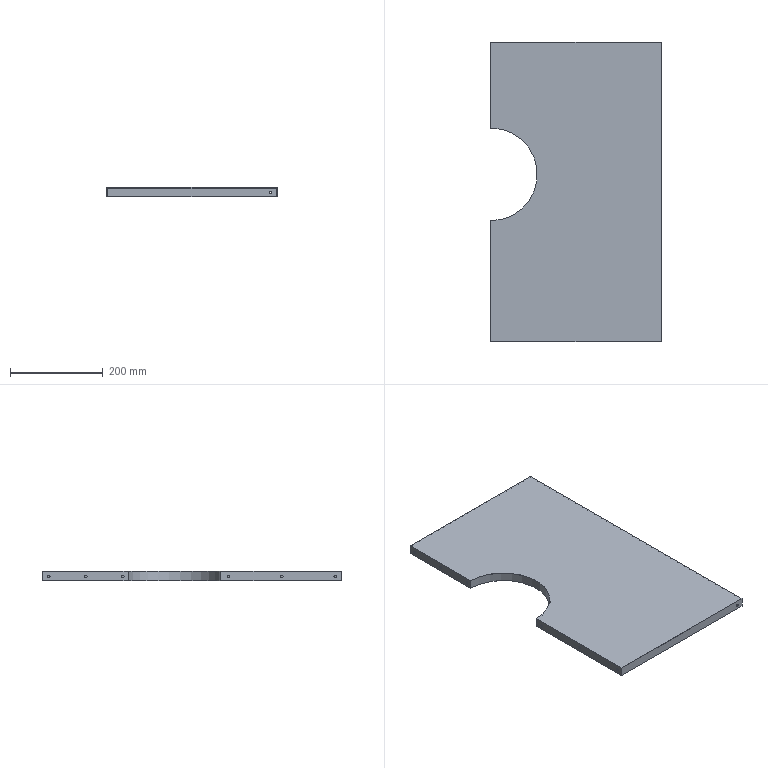Part | SolidWorks | features ICE 2, Extrusion 1, Shell 1 | 1 solid | 31 faces | box 367 x 646 x 20 mm | volume 519095 mm3 | cylinder 18 | plane 13 | commonest cylinder face diameters 5.5 x16 200 x1 204 x1
STEP:
#1=CARTESIAN_POINT('',(0.,244.,11.75));
#2=VERTEX_POINT('',#1);
#3=CARTESIAN_POINT('',(0.,244.,6.25));
#4=VERTEX_POINT('',#3);
#5=CARTESIAN_POINT('',(0.,244.,9.));
#6=DIRECTION('',(1.,0.,0.));
#7=DIRECTION('',(0.,0.,-1.));
#8=AXIS2_PLACEMENT_3D('',#5,#6,#7);
#9=CIRCLE('',#8,2.75);
#10=EDGE_CURVE('',#2,#4,#9,.T.);
#11=ORIENTED_EDGE('',*,*,#10,.F.);
#12=CARTESIAN_POINT('',(2.,244.,11.75));
#13=VERTEX_POINT('',#12);
#14=CARTESIAN_POINT('',(-8.,244.,11.75));
#15=DIRECTION('',(1.,0.,0.));
#16=VECTOR('',#15,1000.);
#17=LINE('',#14,#16);
#18=EDGE_CURVE('',#2,#13,#17,.T.);
#19=ORIENTED_EDGE('',*,*,#18,.T.);
#20=CARTESIAN_POINT('',(2.,244.,6.25));
#21=VERTEX_POINT('',#20);
#22=CARTESIAN_POINT('',(2.,244.,9.));
#23=DIRECTION('',(1.,0.,0.));
#24=DIRECTION('',(0.,0.,-1.));
#25=AXIS2_PLACEMENT_3D('',#22,#23,#24);
#26=CIRCLE('',#25,2.75);
#27=EDGE_CURVE('',#13,#21,#26,.T.);
#28=ORIENTED_EDGE('',*,*,#27,.T.);
#29=CARTESIAN_POINT('',(-8.,244.,6.25));
#30=DIRECTION('',(1.,0.,0.));
#31=VECTOR('',#30,1000.);
#32=LINE('',#29,#31);
#33=EDGE_CURVE('',#4,#21,#32,.T.);
#34=ORIENTED_EDGE('',*,*,#33,.F.);
#35=EDGE_LOOP('',(#11,#19,#28,#34));
#36=FACE_OUTER_BOUND('',#35,.T.);
#37=CARTESIAN_POINT('',(-8.,244.,9.));
#38=DIRECTION('',(1.,0.,0.));
#39=DIRECTION('',(0.,0.,-1.));
#40=AXIS2_PLACEMENT_3D('',#37,#38,#39);
#41=CYLINDRICAL_SURFACE('',#40,2.75);
#42=ADVANCED_FACE('',(#36),#41,.F.);
#43=CARTESIAN_POINT('',(0.,129.,11.75));
#44=VERTEX_POINT('',#43);
#45=CARTESIAN_POINT('',(0.,129.,6.25));
#46=VERTEX_POINT('',#45);
#47=CARTESIAN_POINT('',(0.,129.,9.));
#48=DIRECTION('',(1.,0.,0.));
#49=DIRECTION('',(0.,0.,-1.));
#50=AXIS2_PLACEMENT_3D('',#47,#48,#49);
#51=CIRCLE('',#50,2.75);
#52=EDGE_CURVE('',#44,#46,#51,.T.);
#53=ORIENTED_EDGE('',*,*,#52,.F.);
#54=CARTESIAN_POINT('',(2.,129.,11.75));
#55=VERTEX_POINT('',#54);
#56=CARTESIAN_POINT('',(-8.,129.,11.75));
#57=DIRECTION('',(1.,0.,0.));
#58=VECTOR('',#57,1000.);
#59=LINE('',#56,#58);
#60=EDGE_CURVE('',#44,#55,#59,.T.);
#61=ORIENTED_EDGE('',*,*,#60,.T.);
#62=CARTESIAN_POINT('',(2.,129.,6.25));
#63=VERTEX_POINT('',#62);
#64=CARTESIAN_POINT('',(2.,129.,9.));
#65=DIRECTION('',(1.,0.,0.));
#66=DIRECTION('',(0.,0.,-1.));
#67=AXIS2_PLACEMENT_3D('',#64,#65,#66);
#68=CIRCLE('',#67,2.75);
#69=EDGE_CURVE('',#55,#63,#68,.T.);
#70=ORIENTED_EDGE('',*,*,#69,.T.);
#71=CARTESIAN_POINT('',(-8.,129.,6.25));
#72=DIRECTION('',(1.,0.,0.));
#73=VECTOR('',#72,1000.);
#74=LINE('',#71,#73);
#75=EDGE_CURVE('',#46,#63,#74,.T.);
#76=ORIENTED_EDGE('',*,*,#75,.F.);
#77=EDGE_LOOP('',(#53,#61,#70,#76));
#78=FACE_OUTER_BOUND('',#77,.T.);
#79=CARTESIAN_POINT('',(-8.,129.,9.));
#80=DIRECTION('',(1.,0.,0.));
#81=DIRECTION('',(0.,0.,-1.));
#82=AXIS2_PLACEMENT_3D('',#79,#80,#81);
#83=CYLINDRICAL_SURFACE('',#82,2.75);
#84=ADVANCED_FACE('',(#78),#83,.F.);
#85=CARTESIAN_POINT('',(0.,14.,11.75));
#86=VERTEX_POINT('',#85);
#87=CARTESIAN_POINT('',(0.,14.,6.25));
#88=VERTEX_POINT('',#87);
#89=CARTESIAN_POINT('',(0.,14.,9.));
#90=DIRECTION('',(1.,0.,0.));
#91=DIRECTION('',(0.,0.,-1.));
#92=AXIS2_PLACEMENT_3D('',#89,#90,#91);
#93=CIRCLE('',#92,2.75);
#94=EDGE_CURVE('',#86,#88,#93,.T.);
#95=ORIENTED_EDGE('',*,*,#94,.F.);
#96=CARTESIAN_POINT('',(2.,14.,11.75));
#97=VERTEX_POINT('',#96);
#98=CARTESIAN_POINT('',(-8.,14.,11.75));
#99=DIRECTION('',(1.,0.,0.));
#100=VECTOR('',#99,1000.);
#101=LINE('',#98,#100);
#102=EDGE_CURVE('',#86,#97,#101,.T.);
#103=ORIENTED_EDGE('',*,*,#102,.T.);
#104=CARTESIAN_POINT('',(2.,14.,6.25));
#105=VERTEX_POINT('',#104);
#106=CARTESIAN_POINT('',(2.,14.,9.));
#107=DIRECTION('',(1.,0.,0.));
#108=DIRECTION('',(0.,0.,-1.));
#109=AXIS2_PLACEMENT_3D('',#106,#107,#108);
#110=CIRCLE('',#109,2.75);
#111=EDGE_CURVE('',#97,#105,#110,.T.);
#112=ORIENTED_EDGE('',*,*,#111,.T.);
#113=CARTESIAN_POINT('',(-8.,14.,6.25));
#114=DIRECTION('',(1.,0.,0.));
#115=VECTOR('',#114,1000.);
#116=LINE('',#113,#115);
#117=EDGE_CURVE('',#88,#105,#116,.T.);
#118=ORIENTED_EDGE('',*,*,#117,.F.);
#119=EDGE_LOOP('',(#95,#103,#112,#118));
#120=FACE_OUTER_BOUND('',#119,.T.);
#121=CARTESIAN_POINT('',(-8.,14.,9.));
#122=DIRECTION('',(1.,0.,0.));
#123=DIRECTION('',(0.,0.,-1.));
#124=AXIS2_PLACEMENT_3D('',#121,#122,#123);
#125=CYLINDRICAL_SURFACE('',#124,2.75);
#126=ADVANCED_FACE('',(#120),#125,.F.);
#127=CARTESIAN_POINT('',(0.,472.,11.75));
#128=VERTEX_POINT('',#127);
#129=CARTESIAN_POINT('',(0.,472.,6.25));
#130=VERTEX_POINT('',#129);
#131=CARTESIAN_POINT('',(0.,472.,9.));
#132=DIRECTION('',(1.,0.,0.));
#133=DIRECTION('',(0.,0.,-1.));
#134=AXIS2_PLACEMENT_3D('',#131,#132,#133);
#135=CIRCLE('',#134,2.75);
#136=EDGE_CURVE('',#128,#130,#135,.T.);
#137=ORIENTED_EDGE('',*,*,#136,.F.);
#138=CARTESIAN_POINT('',(2.,472.,11.75));
#139=VERTEX_POINT('',#138);
#140=CARTESIAN_POINT('',(-8.,472.,11.75));
#141=DIRECTION('',(1.,0.,0.));
#142=VECTOR('',#141,1000.);
#143=LINE('',#140,#142);
#144=EDGE_CURVE('',#128,#139,#143,.T.);
#145=ORIENTED_EDGE('',*,*,#144,.T.);
#146=CARTESIAN_POINT('',(2.,472.,6.25));
#147=VERTEX_POINT('',#146);
#148=CARTESIAN_POINT('',(2.,472.,9.));
#149=DIRECTION('',(1.,0.,0.));
#150=DIRECTION('',(0.,0.,-1.));
#151=AXIS2_PLACEMENT_3D('',#148,#149,#150);
#152=CIRCLE('',#151,2.75);
#153=EDGE_CURVE('',#139,#147,#152,.T.);
#154=ORIENTED_EDGE('',*,*,#153,.T.);
#155=CARTESIAN_POINT('',(-8.,472.,6.25));
#156=DIRECTION('',(1.,0.,0.));
#157=VECTOR('',#156,1000.);
#158=LINE('',#155,#157);
#159=EDGE_CURVE('',#130,#147,#158,.T.);
#160=ORIENTED_EDGE('',*,*,#159,.F.);
#161=EDGE_LOOP('',(#137,#145,#154,#160));
#162=FACE_OUTER_BOUND('',#161,.T.);
#163=CARTESIAN_POINT('',(-8.,472.,9.));
#164=DIRECTION('',(1.,0.,0.));
#165=DIRECTION('',(0.,0.,-1.));
#166=AXIS2_PLACEMENT_3D('',#163,#164,#165);
#167=CYLINDRICAL_SURFACE('',#166,2.75);
#168=ADVANCED_FACE('',(#162),#167,.F.);
#169=CARTESIAN_POINT('',(0.,552.,11.75));
#170=VERTEX_POINT('',#169);
#171=CARTESIAN_POINT('',(0.,552.,6.25));
#172=VERTEX_POINT('',#171);
#173=CARTESIAN_POINT('',(0.,552.,9.));
#174=DIRECTION('',(1.,0.,0.));
#175=DIRECTION('',(0.,0.,-1.));
#176=AXIS2_PLACEMENT_3D('',#173,#174,#175);
#177=CIRCLE('',#176,2.75);
#178=EDGE_CURVE('',#170,#172,#177,.T.);
#179=ORIENTED_EDGE('',*,*,#178,.F.);
#180=CARTESIAN_POINT('',(2.,552.,11.75));
#181=VERTEX_POINT('',#180);
#182=CARTESIAN_POINT('',(-8.,552.,11.75));
#183=DIRECTION('',(1.,0.,0.));
#184=VECTOR('',#183,1000.);
#185=LINE('',#182,#184);
#186=EDGE_CURVE('',#170,#181,#185,.T.);
#187=ORIENTED_EDGE('',*,*,#186,.T.);
#188=CARTESIAN_POINT('',(2.,552.,6.25));
#189=VERTEX_POINT('',#188);
#190=CARTESIAN_POINT('',(2.,552.,9.));
#191=DIRECTION('',(1.,0.,0.));
#192=DIRECTION('',(0.,0.,-1.));
#193=AXIS2_PLACEMENT_3D('',#190,#191,#192);
#194=CIRCLE('',#193,2.75);
#195=EDGE_CURVE('',#181,#189,#194,.T.);
#196=ORIENTED_EDGE('',*,*,#195,.T.);
#197=CARTESIAN_POINT('',(-8.,552.,6.25));
#198=DIRECTION('',(1.,0.,0.));
#199=VECTOR('',#198,1000.);
#200=LINE('',#197,#199);
#201=EDGE_CURVE('',#172,#189,#200,.T.);
#202=ORIENTED_EDGE('',*,*,#201,.F.);
#203=EDGE_LOOP('',(#179,#187,#196,#202));
#204=FACE_OUTER_BOUND('',#203,.T.);
#205=CARTESIAN_POINT('',(-8.,552.,9.));
#206=DIRECTION('',(1.,0.,0.));
#207=DIRECTION('',(0.,0.,-1.));
#208=AXIS2_PLACEMENT_3D('',#205,#206,#207);
#209=CYLINDRICAL_SURFACE('',#208,2.75);
#210=ADVANCED_FACE('',(#204),#209,.F.);
#211=CARTESIAN_POINT('',(0.,632.,11.75));
#212=VERTEX_POINT('',#211);
#213=CARTESIAN_POINT('',(0.,632.,6.25));
#214=VERTEX_POINT('',#213);
#215=CARTESIAN_POINT('',(0.,632.,9.));
#216=DIRECTION('',(1.,0.,0.));
#217=DIRECTION('',(0.,0.,-1.));
#218=AXIS2_PLACEMENT_3D('',#215,#216,#217);
#219=CIRCLE('',#218,2.75);
#220=EDGE_CURVE('',#212,#214,#219,.T.);
#221=ORIENTED_EDGE('',*,*,#220,.F.);
#222=CARTESIAN_POINT('',(2.,632.,11.75));
#223=VERTEX_POINT('',#222);
#224=CARTESIAN_POINT('',(-8.,632.,11.75));
#225=DIRECTION('',(1.,0.,0.));
#226=VECTOR('',#225,1000.);
#227=LINE('',#224,#226);
#228=EDGE_CURVE('',#212,#223,#227,.T.);
#229=ORIENTED_EDGE('',*,*,#228,.T.);
#230=CARTESIAN_POINT('',(2.,632.,6.25));
#231=VERTEX_POINT('',#230);
#232=CARTESIAN_POINT('',(2.,632.,9.));
#233=DIRECTION('',(1.,0.,0.));
#234=DIRECTION('',(0.,0.,-1.));
#235=AXIS2_PLACEMENT_3D('',#232,#233,#234);
#236=CIRCLE('',#235,2.75);
#237=EDGE_CURVE('',#223,#231,#236,.T.);
#238=ORIENTED_EDGE('',*,*,#237,.T.);
#239=CARTESIAN_POINT('',(-8.,632.,6.25));
#240=DIRECTION('',(1.,0.,0.));
#241=VECTOR('',#240,1000.);
#242=LINE('',#239,#241);
#243=EDGE_CURVE('',#214,#231,#242,.T.);
#244=ORIENTED_EDGE('',*,*,#243,.F.);
#245=EDGE_LOOP('',(#221,#229,#238,#244));
#246=FACE_OUTER_BOUND('',#245,.T.);
#247=CARTESIAN_POINT('',(-8.,632.,9.));
#248=DIRECTION('',(1.,0.,0.));
#249=DIRECTION('',(0.,0.,-1.));
#250=AXIS2_PLACEMENT_3D('',#247,#248,#249);
#251=CYLINDRICAL_SURFACE('',#250,2.75);
#252=ADVANCED_FACE('',(#246),#251,.F.);
#253=CARTESIAN_POINT('',(353.,2.,11.75));
#254=VERTEX_POINT('',#253);
#255=CARTESIAN_POINT('',(353.,2.,6.25));
#256=VERTEX_POINT('',#255);
#257=CARTESIAN_POINT('',(353.,2.,9.));
#258=DIRECTION('',(0.,-1.,0.));
#259=DIRECTION('',(0.,0.,1.));
#260=AXIS2_PLACEMENT_3D('',#257,#258,#259);
#261=CIRCLE('',#260,2.75);
#262=EDGE_CURVE('',#254,#256,#261,.T.);
#263=ORIENTED_EDGE('',*,*,#262,.F.);
#264=CARTESIAN_POINT('',(353.,0.,11.75));
#265=VERTEX_POINT('',#264);
#266=CARTESIAN_POINT('',(353.,794.,11.75));
#267=DIRECTION('',(0.,-1.,0.));
#268=VECTOR('',#267,1000.);
#269=LINE('',#266,#268);
#270=EDGE_CURVE('',#254,#265,#269,.T.);
#271=ORIENTED_EDGE('',*,*,#270,.T.);
#272=CARTESIAN_POINT('',(353.,0.,6.25));
#273=VERTEX_POINT('',#272);
#274=CARTESIAN_POINT('',(353.,0.,9.));
#275=DIRECTION('',(0.,-1.,0.));
#276=DIRECTION('',(0.,0.,1.));
#277=AXIS2_PLACEMENT_3D('',#274,#275,#276);
#278=CIRCLE('',#277,2.75);
#279=EDGE_CURVE('',#265,#273,#278,.T.);
#280=ORIENTED_EDGE('',*,*,#279,.T.);
#281=CARTESIAN_POINT('',(353.,794.,6.25));
#282=DIRECTION('',(0.,-1.,0.));
#283=VECTOR('',#282,1000.);
#284=LINE('',#281,#283);
#285=EDGE_CURVE('',#256,#273,#284,.T.);
#286=ORIENTED_EDGE('',*,*,#285,.F.);
#287=EDGE_LOOP('',(#263,#271,#280,#286));
#288=FACE_OUTER_BOUND('',#287,.T.);
#289=CARTESIAN_POINT('',(353.,794.,9.));
#290=DIRECTION('',(0.,-1.,0.));
#291=DIRECTION('',(0.,0.,-1.));
#292=AXIS2_PLACEMENT_3D('',#289,#290,#291);
#293=CYLINDRICAL_SURFACE('',#292,2.75);
#294=ADVANCED_FACE('',(#288),#293,.F.);
#295=CARTESIAN_POINT('',(353.,646.,6.25));
#296=VERTEX_POINT('',#295);
#297=CARTESIAN_POINT('',(353.,646.,11.75));
#298=VERTEX_POINT('',#297);
#299=CARTESIAN_POINT('',(353.,646.,9.));
#300=DIRECTION('',(0.,1.,0.));
#301=DIRECTION('',(0.,0.,-1.));
#302=AXIS2_PLACEMENT_3D('',#299,#300,#301);
#303=CIRCLE('',#302,2.75);
#304=EDGE_CURVE('',#296,#298,#303,.T.);
#305=ORIENTED_EDGE('',*,*,#304,.T.);
#306=CARTESIAN_POINT('',(353.,644.,11.75));
#307=VERTEX_POINT('',#306);
#308=CARTESIAN_POINT('',(353.,794.,11.75));
#309=DIRECTION('',(0.,-1.,0.));
#310=VECTOR('',#309,1000.);
#311=LINE('',#308,#310);
#312=EDGE_CURVE('',#298,#307,#311,.T.);
#313=ORIENTED_EDGE('',*,*,#312,.T.);
#314=CARTESIAN_POINT('',(353.,644.,6.25));
#315=VERTEX_POINT('',#314);
#316=CARTESIAN_POINT('',(353.,644.,9.));
#317=DIRECTION('',(0.,1.,0.));
#318=DIRECTION('',(0.,0.,-1.));
#319=AXIS2_PLACEMENT_3D('',#316,#317,#318);
#320=CIRCLE('',#319,2.75);
#321=EDGE_CURVE('',#315,#307,#320,.T.);
#322=ORIENTED_EDGE('',*,*,#321,.F.);
#323=CARTESIAN_POINT('',(353.,794.,6.25));
#324=DIRECTION('',(0.,-1.,0.));
#325=VECTOR('',#324,1000.);
#326=LINE('',#323,#325);
#327=EDGE_CURVE('',#296,#315,#326,.T.);
#328=ORIENTED_EDGE('',*,*,#327,.F.);
#329=EDGE_LOOP('',(#305,#313,#322,#328));
#330=FACE_OUTER_BOUND('',#329,.T.);
#331=CARTESIAN_POINT('',(353.,794.,9.));
#332=DIRECTION('',(0.,-1.,0.));
#333=DIRECTION('',(0.,0.,-1.));
#334=AXIS2_PLACEMENT_3D('',#331,#332,#333);
#335=CYLINDRICAL_SURFACE('',#334,2.75);
#336=ADVANCED_FACE('',(#330),#335,.F.);
#337=CARTESIAN_POINT('',(0.,0.,0.));
#338=VERTEX_POINT('',#337);
#339=CARTESIAN_POINT('',(367.,0.,0.));
#340=VERTEX_POINT('',#339);
#341=CARTESIAN_POINT('',(0.,0.,0.));
#342=DIRECTION('',(1.,0.,0.));
#343=VECTOR('',#342,1000.);
#344=LINE('',#341,#343);
#345=EDGE_CURVE('',#338,#340,#344,.T.);
#346=ORIENTED_EDGE('',*,*,#345,.T.);
#347=CARTESIAN_POINT('',(367.,0.,20.));
#348=VERTEX_POINT('',#347);
#349=CARTESIAN_POINT('',(367.,0.,20.));
#350=DIRECTION('',(0.,0.,-1.));
#351=VECTOR('',#350,1000.);
#352=LINE('',#349,#351);
#353=EDGE_CURVE('',#348,#340,#352,.T.);
#354=ORIENTED_EDGE('',*,*,#353,.F.);
#355=CARTESIAN_POINT('',(0.,0.,20.));
#356=VERTEX_POINT('',#355);
#357=CARTESIAN_POINT('',(0.,0.,20.));
#358=DIRECTION('',(1.,0.,0.));
#359=VECTOR('',#358,1000.);
#360=LINE('',#357,#359);
#361=EDGE_CURVE('',#356,#348,#360,.T.);
#362=ORIENTED_EDGE('',*,*,#361,.F.);
#363=CARTESIAN_POINT('',(0.,0.,20.));
#364=DIRECTION('',(0.,0.,-1.));
#365=VECTOR('',#364,1000.);
#366=LINE('',#363,#365);
#367=EDGE_CURVE('',#356,#338,#366,.T.);
#368=ORIENTED_EDGE('',*,*,#367,.T.);
#369=EDGE_LOOP('',(#346,#354,#362,#368));
#370=FACE_OUTER_BOUND('',#369,.T.);
#371=CARTESIAN_POINT('',(353.,0.,9.));
#372=DIRECTION('',(0.,-1.,0.));
#373=DIRECTION('',(0.,0.,1.));
#374=AXIS2_PLACEMENT_3D('',#371,#372,#373);
#375=CIRCLE('',#374,2.75);
#376=EDGE_CURVE('',#273,#265,#375,.T.);
#377=ORIENTED_EDGE('',*,*,#376,.F.);
#378=ORIENTED_EDGE('',*,*,#279,.F.);
#379=EDGE_LOOP('',(#377,#378));
#380=FACE_BOUND('',#379,.T.);
#381=CARTESIAN_POINT('',(0.,0.,20.));
#382=DIRECTION('',(0.,1.,0.));
#383=DIRECTION('',(0.,0.,1.));
#384=AXIS2_PLACEMENT_3D('',#381,#382,#383);
#385=PLANE('',#384);
#386=ADVANCED_FACE('',(#370,#380),#385,.F.);
#387=CARTESIAN_POINT('',(367.,646.,0.));
#388=VERTEX_POINT('',#387);
#389=CARTESIAN_POINT('',(0.,646.,0.));
#390=VERTEX_POINT('',#389);
#391=CARTESIAN_POINT('',(0.,646.,0.));
#392=DIRECTION('',(-1.,0.,0.));
#393=VECTOR('',#392,1000.);
#394=LINE('',#391,#393);
#395=EDGE_CURVE('',#388,#390,#394,.T.);
#396=ORIENTED_EDGE('',*,*,#395,.T.);
#397=CARTESIAN_POINT('',(0.,646.,20.));
#398=VERTEX_POINT('',#397);
#399=CARTESIAN_POINT('',(0.,646.,20.));
#400=DIRECTION('',(0.,0.,-1.));
#401=VECTOR('',#400,1000.);
#402=LINE('',#399,#401);
#403=EDGE_CURVE('',#398,#390,#402,.T.);
#404=ORIENTED_EDGE('',*,*,#403,.F.);
#405=CARTESIAN_POINT('',(367.,646.,20.));
#406=VERTEX_POINT('',#405);
#407=CARTESIAN_POINT('',(0.,646.,20.));
#408=DIRECTION('',(-1.,0.,0.));
#409=VECTOR('',#408,1000.);
#410=LINE('',#407,#409);
#411=EDGE_CURVE('',#406,#398,#410,.T.);
#412=ORIENTED_EDGE('',*,*,#411,.F.);
#413=CARTESIAN_POINT('',(367.,646.,20.));
#414=DIRECTION('',(0.,0.,-1.));
#415=VECTOR('',#414,1000.);
#416=LINE('',#413,#415);
#417=EDGE_CURVE('',#406,#388,#416,.T.);
#418=ORIENTED_EDGE('',*,*,#417,.T.);
#419=EDGE_LOOP('',(#396,#404,#412,#418));
#420=FACE_OUTER_BOUND('',#419,.T.);
#421=ORIENTED_EDGE('',*,*,#304,.F.);
#422=CARTESIAN_POINT('',(353.,646.,9.));
#423=DIRECTION('',(0.,1.,0.));
#424=DIRECTION('',(0.,0.,-1.));
#425=AXIS2_PLACEMENT_3D('',#422,#423,#424);
#426=CIRCLE('',#425,2.75);
#427=EDGE_CURVE('',#298,#296,#426,.T.);
#428=ORIENTED_EDGE('',*,*,#427,.F.);
#429=EDGE_LOOP('',(#421,#428));
#430=FACE_BOUND('',#429,.T.);
#431=CARTESIAN_POINT('',(0.,646.,20.));
#432=DIRECTION('',(0.,-1.,0.));
#433=DIRECTION('',(0.,0.,-1.));
#434=AXIS2_PLACEMENT_3D('',#431,#432,#433);
#435=PLANE('',#434);
#436=ADVANCED_FACE('',(#420,#430),#435,.F.);
#437=CARTESIAN_POINT('',(2.,2.,0.));
#438=VERTEX_POINT('',#437);
#439=CARTESIAN_POINT('',(365.,2.,0.));
#440=VERTEX_POINT('',#439);
#441=CARTESIAN_POINT('',(0.,2.,0.));
#442=DIRECTION('',(1.,0.,0.));
#443=VECTOR('',#442,1000.);
#444=LINE('',#441,#443);
#445=EDGE_CURVE('',#438,#440,#444,.T.);
#446=ORIENTED_EDGE('',*,*,#445,.F.);
#447=CARTESIAN_POINT('',(2.,2.,18.));
#448=VERTEX_POINT('',#447);
#449=CARTESIAN_POINT('',(2.,2.,20.));
#450=DIRECTION('',(0.,0.,-1.));
#451=VECTOR('',#450,1000.);
#452=LINE('',#449,#451);
#453=EDGE_CURVE('',#448,#438,#452,.T.);
#454=ORIENTED_EDGE('',*,*,#453,.F.);
#455=CARTESIAN_POINT('',(365.,2.,18.));
#456=VERTEX_POINT('',#455);
#457=CARTESIAN_POINT('',(0.,2.,18.));
#458=DIRECTION('',(1.,0.,0.));
#459=VECTOR('',#458,1000.);
#460=LINE('',#457,#459);
#461=EDGE_CURVE('',#448,#456,#460,.T.);
#462=ORIENTED_EDGE('',*,*,#461,.T.);
#463=CARTESIAN_POINT('',(365.,2.,20.));
#464=DIRECTION('',(0.,0.,-1.));
#465=VECTOR('',#464,1000.);
#466=LINE('',#463,#465);
#467=EDGE_CURVE('',#456,#440,#466,.T.);
#468=ORIENTED_EDGE('',*,*,#467,.T.);
#469=EDGE_LOOP('',(#446,#454,#462,#468));
#470=FACE_OUTER_BOUND('',#469,.T.);
#471=CARTESIAN_POINT('',(353.,2.,9.));
#472=DIRECTION('',(0.,-1.,0.));
#473=DIRECTION('',(0.,0.,1.));
#474=AXIS2_PLACEMENT_3D('',#471,#472,#473);
#475=CIRCLE('',#474,2.75);
#476=EDGE_CURVE('',#256,#254,#475,.T.);
#477=ORIENTED_EDGE('',*,*,#476,.T.);
#478=ORIENTED_EDGE('',*,*,#262,.T.);
#479=EDGE_LOOP('',(#477,#478));
#480=FACE_BOUND('',#479,.T.);
#481=CARTESIAN_POINT('',(0.,2.,20.));
#482=DIRECTION('',(0.,1.,0.));
#483=DIRECTION('',(0.,0.,1.));
#484=AXIS2_PLACEMENT_3D('',#481,#482,#483);
#485=PLANE('',#484);
#486=ADVANCED_FACE('',(#470,#480),#485,.T.);
#487=CARTESIAN_POINT('',(365.,644.,0.));
#488=VERTEX_POINT('',#487);
#489=CARTESIAN_POINT('',(2.,644.,0.));
#490=VERTEX_POINT('',#489);
#491=CARTESIAN_POINT('',(0.,644.,0.));
#492=DIRECTION('',(-1.,0.,0.));
#493=VECTOR('',#492,1000.);
#494=LINE('',#491,#493);
#495=EDGE_CURVE('',#488,#490,#494,.T.);
#496=ORIENTED_EDGE('',*,*,#495,.F.);
#497=CARTESIAN_POINT('',(365.,644.,18.));
#498=VERTEX_POINT('',#497);
#499=CARTESIAN_POINT('',(365.,644.,20.));
#500=DIRECTION('',(0.,0.,-1.));
#501=VECTOR('',#500,1000.);
#502=LINE('',#499,#501);
#503=EDGE_CURVE('',#498,#488,#502,.T.);
#504=ORIENTED_EDGE('',*,*,#503,.F.);
#505=CARTESIAN_POINT('',(2.,644.,18.));
#506=VERTEX_POINT('',#505);
#507=CARTESIAN_POINT('',(0.,644.,18.));
#508=DIRECTION('',(-1.,0.,0.));
#509=VECTOR('',#508,1000.);
#510=LINE('',#507,#509);
#511=EDGE_CURVE('',#498,#506,#510,.T.);
#512=ORIENTED_EDGE('',*,*,#511,.T.);
#513=CARTESIAN_POINT('',(2.,644.,20.));
#514=DIRECTION('',(0.,0.,-1.));
#515=VECTOR('',#514,1000.);
#516=LINE('',#513,#515);
#517=EDGE_CURVE('',#506,#490,#516,.T.);
#518=ORIENTED_EDGE('',*,*,#517,.T.);
#519=EDGE_LOOP('',(#496,#504,#512,#518));
#520=FACE_OUTER_BOUND('',#519,.T.);
#521=ORIENTED_EDGE('',*,*,#321,.T.);
#522=CARTESIAN_POINT('',(353.,644.,9.));
#523=DIRECTION('',(0.,1.,0.));
#524=DIRECTION('',(0.,0.,-1.));
#525=AXIS2_PLACEMENT_3D('',#522,#523,#524);
#526=CIRCLE('',#525,2.75);
#527=EDGE_CURVE('',#307,#315,#526,.T.);
#528=ORIENTED_EDGE('',*,*,#527,.T.);
#529=EDGE_LOOP('',(#521,#528));
#530=FACE_BOUND('',#529,.T.);
#531=CARTESIAN_POINT('',(0.,644.,20.));
#532=DIRECTION('',(0.,-1.,0.));
#533=DIRECTION('',(0.,0.,-1.));
#534=AXIS2_PLACEMENT_3D('',#531,#532,#533);
#535=PLANE('',#534);
#536=ADVANCED_FACE('',(#520,#530),#535,.T.);
#537=CARTESIAN_POINT('',(0.,244.,9.));
#538=DIRECTION('',(1.,0.,0.));
#539=DIRECTION('',(0.,0.,-1.));
#540=AXIS2_PLACEMENT_3D('',#537,#538,#539);
#541=CIRCLE('',#540,2.75);
#542=EDGE_CURVE('',#4,#2,#541,.T.);
#543=ORIENTED_EDGE('',*,*,#542,.T.);
#544=ORIENTED_EDGE('',*,*,#10,.T.);
#545=EDGE_LOOP('',(#543,#544));
#546=FACE_BOUND('',#545,.T.);
#547=CARTESIAN_POINT('',(0.,129.,9.));
#548=DIRECTION('',(1.,0.,0.));
#549=DIRECTION('',(0.,0.,-1.));
#550=AXIS2_PLACEMENT_3D('',#547,#548,#549);
#551=CIRCLE('',#550,2.75);
#552=EDGE_CURVE('',#46,#44,#551,.T.);
#553=ORIENTED_EDGE('',*,*,#552,.T.);
#554=ORIENTED_EDGE('',*,*,#52,.T.);
#555=EDGE_LOOP('',(#553,#554));
#556=FACE_BOUND('',#555,.T.);
#557=CARTESIAN_POINT('',(0.,14.,9.));
#558=DIRECTION('',(1.,0.,0.));
#559=DIRECTION('',(0.,0.,-1.));
#560=AXIS2_PLACEMENT_3D('',#557,#558,#559);
#561=CIRCLE('',#560,2.75);
#562=EDGE_CURVE('',#88,#86,#561,.T.);
#563=ORIENTED_EDGE('',*,*,#562,.T.);
#564=ORIENTED_EDGE('',*,*,#94,.T.);
#565=EDGE_LOOP('',(#563,#564));
#566=FACE_BOUND('',#565,.T.);
#567=CARTESIAN_POINT('',(0.,261.,0.));
#568=VERTEX_POINT('',#567);
#569=CARTESIAN_POINT('',(0.,0.,0.));
#570=DIRECTION('',(0.,-1.,0.));
#571=VECTOR('',#570,1000.);
#572=LINE('',#569,#571);
#573=EDGE_CURVE('',#568,#338,#572,.T.);
#574=ORIENTED_EDGE('',*,*,#573,.T.);
#575=ORIENTED_EDGE('',*,*,#367,.F.);
#576=CARTESIAN_POINT('',(0.,261.,20.));
#577=VERTEX_POINT('',#576);
#578=CARTESIAN_POINT('',(0.,0.,20.));
#579=DIRECTION('',(0.,-1.,0.));
#580=VECTOR('',#579,1000.);
#581=LINE('',#578,#580);
#582=EDGE_CURVE('',#577,#356,#581,.T.);
#583=ORIENTED_EDGE('',*,*,#582,.F.);
#584=CARTESIAN_POINT('',(0.,261.,20.));
#585=DIRECTION('',(0.,0.,-1.));
#586=VECTOR('',#585,1000.);
#587=LINE('',#584,#586);
#588=EDGE_CURVE('',#577,#568,#587,.T.);
#589=ORIENTED_EDGE('',*,*,#588,.T.);
#590=EDGE_LOOP('',(#574,#575,#583,#589));
#591=FACE_OUTER_BOUND('',#590,.T.);
#592=CARTESIAN_POINT('',(0.,0.,20.));
#593=DIRECTION('',(1.,0.,0.));
#594=DIRECTION('',(0.,0.,-1.));
#595=AXIS2_PLACEMENT_3D('',#592,#593,#594);
#596=PLANE('',#595);
#597=ADVANCED_FACE('',(#546,#556,#566,#591),#596,.F.);
#598=CARTESIAN_POINT('',(367.,0.,0.));
#599=DIRECTION('',(0.,1.,0.));
#600=VECTOR('',#599,1000.);
#601=LINE('',#598,#600);
#602=EDGE_CURVE('',#340,#388,#601,.T.);
#603=ORIENTED_EDGE('',*,*,#602,.T.);
#604=ORIENTED_EDGE('',*,*,#417,.F.);
#605=CARTESIAN_POINT('',(367.,0.,20.));
#606=DIRECTION('',(0.,1.,0.));
#607=VECTOR('',#606,1000.);
#608=LINE('',#605,#607);
#609=EDGE_CURVE('',#348,#406,#608,.T.);
#610=ORIENTED_EDGE('',*,*,#609,.F.);
#611=ORIENTED_EDGE('',*,*,#353,.T.);
#612=EDGE_LOOP('',(#603,#604,#610,#611));
#613=FACE_OUTER_BOUND('',#612,.T.);
#614=CARTESIAN_POINT('',(367.,0.,20.));
#615=DIRECTION('',(-1.,0.,0.));
#616=DIRECTION('',(0.,0.,1.));
#617=AXIS2_PLACEMENT_3D('',#614,#615,#616);
#618=PLANE('',#617);
#619=ADVANCED_FACE('',(#613),#618,.F.);
#620=CARTESIAN_POINT('',(0.,472.,9.));
#621=DIRECTION('',(1.,0.,0.));
#622=DIRECTION('',(0.,0.,-1.));
#623=AXIS2_PLACEMENT_3D('',#620,#621,#622);
#624=CIRCLE('',#623,2.75);
#625=EDGE_CURVE('',#130,#128,#624,.T.);
#626=ORIENTED_EDGE('',*,*,#625,.T.);
#627=ORIENTED_EDGE('',*,*,#136,.T.);
#628=EDGE_LOOP('',(#626,#627));
#629=FACE_BOUND('',#628,.T.);
#630=CARTESIAN_POINT('',(0.,552.,9.));
#631=DIRECTION('',(1.,0.,0.));
#632=DIRECTION('',(0.,0.,-1.));
#633=AXIS2_PLACEMENT_3D('',#630,#631,#632);
#634=CIRCLE('',#633,2.75);
#635=EDGE_CURVE('',#172,#170,#634,.T.);
#636=ORIENTED_EDGE('',*,*,#635,.T.);
#637=ORIENTED_EDGE('',*,*,#178,.T.);
#638=EDGE_LOOP('',(#636,#637));
#639=FACE_BOUND('',#638,.T.);
#640=CARTESIAN_POINT('',(0.,632.,9.));
#641=DIRECTION('',(1.,0.,0.));
#642=DIRECTION('',(0.,0.,-1.));
#643=AXIS2_PLACEMENT_3D('',#640,#641,#642);
#644=CIRCLE('',#643,2.75);
#645=EDGE_CURVE('',#214,#212,#644,.T.);
#646=ORIENTED_EDGE('',*,*,#645,.T.);
#647=ORIENTED_EDGE('',*,*,#220,.T.);
#648=EDGE_LOOP('',(#646,#647));
#649=FACE_BOUND('',#648,.T.);
#650=CARTESIAN_POINT('',(0.,461.,0.));
#651=VERTEX_POINT('',#650);
#652=CARTESIAN_POINT('',(0.,461.,0.));
#653=DIRECTION('',(0.,-1.,0.));
#654=VECTOR('',#653,1000.);
#655=LINE('',#652,#654);
#656=EDGE_CURVE('',#390,#651,#655,.T.);
#657=ORIENTED_EDGE('',*,*,#656,.T.);
#658=CARTESIAN_POINT('',(0.,461.,20.));
#659=VERTEX_POINT('',#658);
#660=CARTESIAN_POINT('',(0.,461.,20.));
#661=DIRECTION('',(0.,0.,-1.));
#662=VECTOR('',#661,1000.);
#663=LINE('',#660,#662);
#664=EDGE_CURVE('',#659,#651,#663,.T.);
#665=ORIENTED_EDGE('',*,*,#664,.F.);
#666=CARTESIAN_POINT('',(0.,461.,20.));
#667=DIRECTION('',(0.,-1.,0.));
#668=VECTOR('',#667,1000.);
#669=LINE('',#666,#668);
#670=EDGE_CURVE('',#398,#659,#669,.T.);
#671=ORIENTED_EDGE('',*,*,#670,.F.);
#672=ORIENTED_EDGE('',*,*,#403,.T.);
#673=EDGE_LOOP('',(#657,#665,#671,#672));
#674=FACE_OUTER_BOUND('',#673,.T.);
#675=CARTESIAN_POINT('',(0.,461.,20.));
#676=DIRECTION('',(1.,0.,0.));
#677=DIRECTION('',(0.,0.,-1.));
#678=AXIS2_PLACEMENT_3D('',#675,#676,#677);
#679=PLANE('',#678);
#680=ADVANCED_FACE('',(#629,#639,#649,#674),#679,.F.);
#681=CARTESIAN_POINT('',(0.,361.,0.));
#682=DIRECTION('',(0.,0.,-1.));
#683=DIRECTION('',(1.,0.,0.));
#684=AXIS2_PLACEMENT_3D('',#681,#682,#683);
#685=CIRCLE('',#684,100.);
#686=EDGE_CURVE('',#651,#568,#685,.T.);
#687=ORIENTED_EDGE('',*,*,#686,.T.);
#688=ORIENTED_EDGE('',*,*,#588,.F.);
#689=CARTESIAN_POINT('',(0.,361.,20.));
#690=DIRECTION('',(0.,0.,-1.));
#691=DIRECTION('',(1.,0.,0.));
#692=AXIS2_PLACEMENT_3D('',#689,#690,#691);
#693=CIRCLE('',#692,100.);
#694=EDGE_CURVE('',#659,#577,#693,.T.);
#695=ORIENTED_EDGE('',*,*,#694,.F.);
#696=ORIENTED_EDGE('',*,*,#664,.T.);
#697=EDGE_LOOP('',(#687,#688,#695,#696));
#698=FACE_OUTER_BOUND('',#697,.T.);
#699=CARTESIAN_POINT('',(0.,361.,20.));
#700=DIRECTION('',(0.,0.,-1.));
#701=DIRECTION('',(-1.,0.,0.));
#702=AXIS2_PLACEMENT_3D('',#699,#700,#701);
#703=CYLINDRICAL_SURFACE('',#702,100.);
#704=ADVANCED_FACE('',(#698),#703,.F.);
#705=ORIENTED_EDGE('',*,*,#582,.T.);
#706=ORIENTED_EDGE('',*,*,#361,.T.);
#707=ORIENTED_EDGE('',*,*,#609,.T.);
#708=ORIENTED_EDGE('',*,*,#411,.T.);
#709=ORIENTED_EDGE('',*,*,#670,.T.);
#710=ORIENTED_EDGE('',*,*,#694,.T.);
#711=EDGE_LOOP('',(#705,#706,#707,#708,#709,#710));
#712=FACE_OUTER_BOUND('',#711,.T.);
#713=CARTESIAN_POINT('',(0.,361.,20.));
#714=DIRECTION('',(0.,0.,1.));
#715=DIRECTION('',(1.,0.,0.));
#716=AXIS2_PLACEMENT_3D('',#713,#714,#715);
#717=PLANE('',#716);
#718=ADVANCED_FACE('',(#712),#717,.T.);
#719=CARTESIAN_POINT('',(2.,462.98,0.));
#720=VERTEX_POINT('',#719);
#721=CARTESIAN_POINT('',(2.,259.02,0.));
#722=VERTEX_POINT('',#721);
#723=CARTESIAN_POINT('',(0.,361.,0.));
#724=DIRECTION('',(0.,0.,-1.));
#725=DIRECTION('',(1.,0.,0.));
#726=AXIS2_PLACEMENT_3D('',#723,#724,#725);
#727=CIRCLE('',#726,102.);
#728=EDGE_CURVE('',#720,#722,#727,.T.);
#729=ORIENTED_EDGE('',*,*,#728,.T.);
#730=CARTESIAN_POINT('',(2.,0.,0.));
#731=DIRECTION('',(0.,-1.,0.));
#732=VECTOR('',#731,1000.);
#733=LINE('',#730,#732);
#734=EDGE_CURVE('',#722,#438,#733,.T.);
#735=ORIENTED_EDGE('',*,*,#734,.T.);
#736=ORIENTED_EDGE('',*,*,#445,.T.);
#737=CARTESIAN_POINT('',(365.,0.,0.));
#738=DIRECTION('',(0.,1.,0.));
#739=VECTOR('',#738,1000.);
#740=LINE('',#737,#739);
#741=EDGE_CURVE('',#440,#488,#740,.T.);
#742=ORIENTED_EDGE('',*,*,#741,.T.);
#743=ORIENTED_EDGE('',*,*,#495,.T.);
#744=CARTESIAN_POINT('',(2.,461.,0.));
#745=DIRECTION('',(0.,-1.,0.));
#746=VECTOR('',#745,1000.);
#747=LINE('',#744,#746);
#748=EDGE_CURVE('',#490,#720,#747,.T.);
#749=ORIENTED_EDGE('',*,*,#748,.T.);
#750=EDGE_LOOP('',(#729,#735,#736,#742,#743,#749));
#751=FACE_BOUND('',#750,.T.);
#752=ORIENTED_EDGE('',*,*,#573,.F.);
#753=ORIENTED_EDGE('',*,*,#686,.F.);
#754=ORIENTED_EDGE('',*,*,#656,.F.);
#755=ORIENTED_EDGE('',*,*,#395,.F.);
#756=ORIENTED_EDGE('',*,*,#602,.F.);
#757=ORIENTED_EDGE('',*,*,#345,.F.);
#758=EDGE_LOOP('',(#752,#753,#754,#755,#756,#757));
#759=FACE_OUTER_BOUND('',#758,.T.);
#760=CARTESIAN_POINT('',(0.,361.,0.));
#761=DIRECTION('',(0.,0.,1.));
#762=DIRECTION('',(1.,0.,0.));
#763=AXIS2_PLACEMENT_3D('',#760,#761,#762);
#764=PLANE('',#763);
#765=ADVANCED_FACE('',(#751,#759),#764,.F.);
#766=CARTESIAN_POINT('',(2.,244.,9.));
#767=DIRECTION('',(1.,0.,0.));
#768=DIRECTION('',(0.,0.,-1.));
#769=AXIS2_PLACEMENT_3D('',#766,#767,#768);
#770=CIRCLE('',#769,2.75);
#771=EDGE_CURVE('',#21,#13,#770,.T.);
#772=ORIENTED_EDGE('',*,*,#771,.F.);
#773=ORIENTED_EDGE('',*,*,#27,.F.);
#774=EDGE_LOOP('',(#772,#773));
#775=FACE_BOUND('',#774,.T.);
#776=CARTESIAN_POINT('',(2.,129.,9.));
#777=DIRECTION('',(1.,0.,0.));
#778=DIRECTION('',(0.,0.,-1.));
#779=AXIS2_PLACEMENT_3D('',#776,#777,#778);
#780=CIRCLE('',#779,2.75);
#781=EDGE_CURVE('',#63,#55,#780,.T.);
#782=ORIENTED_EDGE('',*,*,#781,.F.);
#783=ORIENTED_EDGE('',*,*,#69,.F.);
#784=EDGE_LOOP('',(#782,#783));
#785=FACE_BOUND('',#784,.T.);
#786=CARTESIAN_POINT('',(2.,14.,9.));
#787=DIRECTION('',(1.,0.,0.));
#788=DIRECTION('',(0.,0.,-1.));
#789=AXIS2_PLACEMENT_3D('',#786,#787,#788);
#790=CIRCLE('',#789,2.75);
#791=EDGE_CURVE('',#105,#97,#790,.T.);
#792=ORIENTED_EDGE('',*,*,#791,.F.);
#793=ORIENTED_EDGE('',*,*,#111,.F.);
#794=EDGE_LOOP('',(#792,#793));
#795=FACE_BOUND('',#794,.T.);
#796=ORIENTED_EDGE('',*,*,#734,.F.);
#797=CARTESIAN_POINT('',(2.,259.02,18.));
#798=VERTEX_POINT('',#797);
#799=CARTESIAN_POINT('',(2.,259.02,18.));
#800=DIRECTION('',(0.,0.,-1.));
#801=VECTOR('',#800,1000.);
#802=LINE('',#799,#801);
#803=EDGE_CURVE('',#798,#722,#802,.T.);
#804=ORIENTED_EDGE('',*,*,#803,.F.);
#805=CARTESIAN_POINT('',(2.,0.,18.));
#806=DIRECTION('',(0.,-1.,0.));
#807=VECTOR('',#806,1000.);
#808=LINE('',#805,#807);
#809=EDGE_CURVE('',#798,#448,#808,.T.);
#810=ORIENTED_EDGE('',*,*,#809,.T.);
#811=ORIENTED_EDGE('',*,*,#453,.T.);
#812=EDGE_LOOP('',(#796,#804,#810,#811));
#813=FACE_OUTER_BOUND('',#812,.T.);
#814=CARTESIAN_POINT('',(2.,0.,20.));
#815=DIRECTION('',(1.,0.,0.));
#816=DIRECTION('',(0.,0.,-1.));
#817=AXIS2_PLACEMENT_3D('',#814,#815,#816);
#818=PLANE('',#817);
#819=ADVANCED_FACE('',(#775,#785,#795,#813),#818,.T.);
#820=ORIENTED_EDGE('',*,*,#741,.F.);
#821=ORIENTED_EDGE('',*,*,#467,.F.);
#822=CARTESIAN_POINT('',(365.,0.,18.));
#823=DIRECTION('',(0.,1.,0.));
#824=VECTOR('',#823,1000.);
#825=LINE('',#822,#824);
#826=EDGE_CURVE('',#456,#498,#825,.T.);
#827=ORIENTED_EDGE('',*,*,#826,.T.);
#828=ORIENTED_EDGE('',*,*,#503,.T.);
#829=EDGE_LOOP('',(#820,#821,#827,#828));
#830=FACE_OUTER_BOUND('',#829,.T.);
#831=CARTESIAN_POINT('',(365.,0.,20.));
#832=DIRECTION('',(-1.,0.,0.));
#833=DIRECTION('',(0.,0.,1.));
#834=AXIS2_PLACEMENT_3D('',#831,#832,#833);
#835=PLANE('',#834);
#836=ADVANCED_FACE('',(#830),#835,.T.);
#837=CARTESIAN_POINT('',(2.,472.,9.));
#838=DIRECTION('',(1.,0.,0.));
#839=DIRECTION('',(0.,0.,-1.));
#840=AXIS2_PLACEMENT_3D('',#837,#838,#839);
#841=CIRCLE('',#840,2.75);
#842=EDGE_CURVE('',#147,#139,#841,.T.);
#843=ORIENTED_EDGE('',*,*,#842,.F.);
#844=ORIENTED_EDGE('',*,*,#153,.F.);
#845=EDGE_LOOP('',(#843,#844));
#846=FACE_BOUND('',#845,.T.);
#847=CARTESIAN_POINT('',(2.,552.,9.));
#848=DIRECTION('',(1.,0.,0.));
#849=DIRECTION('',(0.,0.,-1.));
#850=AXIS2_PLACEMENT_3D('',#847,#848,#849);
#851=CIRCLE('',#850,2.75);
#852=EDGE_CURVE('',#189,#181,#851,.T.);
#853=ORIENTED_EDGE('',*,*,#852,.F.);
#854=ORIENTED_EDGE('',*,*,#195,.F.);
#855=EDGE_LOOP('',(#853,#854));
#856=FACE_BOUND('',#855,.T.);
#857=CARTESIAN_POINT('',(2.,632.,9.));
#858=DIRECTION('',(1.,0.,0.));
#859=DIRECTION('',(0.,0.,-1.));
#860=AXIS2_PLACEMENT_3D('',#857,#858,#859);
#861=CIRCLE('',#860,2.75);
#862=EDGE_CURVE('',#231,#223,#861,.T.);
#863=ORIENTED_EDGE('',*,*,#862,.F.);
#864=ORIENTED_EDGE('',*,*,#237,.F.);
#865=EDGE_LOOP('',(#863,#864));
#866=FACE_BOUND('',#865,.T.);
#867=ORIENTED_EDGE('',*,*,#748,.F.);
#868=ORIENTED_EDGE('',*,*,#517,.F.);
#869=CARTESIAN_POINT('',(2.,462.98,18.));
#870=VERTEX_POINT('',#869);
#871=CARTESIAN_POINT('',(2.,461.,18.));
#872=DIRECTION('',(0.,-1.,0.));
#873=VECTOR('',#872,1000.);
#874=LINE('',#871,#873);
#875=EDGE_CURVE('',#506,#870,#874,.T.);
#876=ORIENTED_EDGE('',*,*,#875,.T.);
#877=CARTESIAN_POINT('',(2.,462.98,18.));
#878=DIRECTION('',(0.,0.,-1.));
#879=VECTOR('',#878,1000.);
#880=LINE('',#877,#879);
#881=EDGE_CURVE('',#870,#720,#880,.T.);
#882=ORIENTED_EDGE('',*,*,#881,.T.);
#883=EDGE_LOOP('',(#867,#868,#876,#882));
#884=FACE_OUTER_BOUND('',#883,.T.);
#885=CARTESIAN_POINT('',(2.,461.,20.));
#886=DIRECTION('',(1.,0.,0.));
#887=DIRECTION('',(0.,0.,-1.));
#888=AXIS2_PLACEMENT_3D('',#885,#886,#887);
#889=PLANE('',#888);
#890=ADVANCED_FACE('',(#846,#856,#866,#884),#889,.T.);
#891=ORIENTED_EDGE('',*,*,#728,.F.);
#892=ORIENTED_EDGE('',*,*,#881,.F.);
#893=CARTESIAN_POINT('',(0.,361.,18.));
#894=DIRECTION('',(0.,0.,-1.));
#895=DIRECTION('',(1.,0.,0.));
#896=AXIS2_PLACEMENT_3D('',#893,#894,#895);
#897=CIRCLE('',#896,102.);
#898=EDGE_CURVE('',#870,#798,#897,.T.);
#899=ORIENTED_EDGE('',*,*,#898,.T.);
#900=ORIENTED_EDGE('',*,*,#803,.T.);
#901=EDGE_LOOP('',(#891,#892,#899,#900));
#902=FACE_OUTER_BOUND('',#901,.T.);
#903=CARTESIAN_POINT('',(0.,361.,20.));
#904=DIRECTION('',(0.,0.,-1.));
#905=DIRECTION('',(-1.,0.,0.));
#906=AXIS2_PLACEMENT_3D('',#903,#904,#905);
#907=CYLINDRICAL_SURFACE('',#906,102.);
#908=ADVANCED_FACE('',(#902),#907,.T.);
#909=ORIENTED_EDGE('',*,*,#809,.F.);
#910=ORIENTED_EDGE('',*,*,#898,.F.);
#911=ORIENTED_EDGE('',*,*,#875,.F.);
#912=ORIENTED_EDGE('',*,*,#511,.F.);
#913=ORIENTED_EDGE('',*,*,#826,.F.);
#914=ORIENTED_EDGE('',*,*,#461,.F.);
#915=EDGE_LOOP('',(#909,#910,#911,#912,#913,#914));
#916=FACE_OUTER_BOUND('',#915,.T.);
#917=CARTESIAN_POINT('',(0.,361.,18.));
#918=DIRECTION('',(0.,0.,1.));
#919=DIRECTION('',(1.,0.,0.));
#920=AXIS2_PLACEMENT_3D('',#917,#918,#919);
#921=PLANE('',#920);
#922=ADVANCED_FACE('',(#916),#921,.F.);
#923=ORIENTED_EDGE('',*,*,#312,.F.);
#924=ORIENTED_EDGE('',*,*,#427,.T.);
#925=ORIENTED_EDGE('',*,*,#327,.T.);
#926=ORIENTED_EDGE('',*,*,#527,.F.);
#927=EDGE_LOOP('',(#923,#924,#925,#926));
#928=FACE_OUTER_BOUND('',#927,.T.);
#929=CARTESIAN_POINT('',(353.,794.,9.));
#930=DIRECTION('',(0.,-1.,0.));
#931=DIRECTION('',(0.,0.,-1.));
#932=AXIS2_PLACEMENT_3D('',#929,#930,#931);
#933=CYLINDRICAL_SURFACE('',#932,2.75);
#934=ADVANCED_FACE('',(#928),#933,.F.);
#935=ORIENTED_EDGE('',*,*,#270,.F.);
#936=ORIENTED_EDGE('',*,*,#476,.F.);
#937=ORIENTED_EDGE('',*,*,#285,.T.);
#938=ORIENTED_EDGE('',*,*,#376,.T.);
#939=EDGE_LOOP('',(#935,#936,#937,#938));
#940=FACE_OUTER_BOUND('',#939,.T.);
#941=CARTESIAN_POINT('',(353.,794.,9.));
#942=DIRECTION('',(0.,-1.,0.));
#943=DIRECTION('',(0.,0.,-1.));
#944=AXIS2_PLACEMENT_3D('',#941,#942,#943);
#945=CYLINDRICAL_SURFACE('',#944,2.75);
#946=ADVANCED_FACE('',(#940),#945,.F.);
#947=ORIENTED_EDGE('',*,*,#228,.F.);
#948=ORIENTED_EDGE('',*,*,#645,.F.);
#949=ORIENTED_EDGE('',*,*,#243,.T.);
#950=ORIENTED_EDGE('',*,*,#862,.T.);
#951=EDGE_LOOP('',(#947,#948,#949,#950));
#952=FACE_OUTER_BOUND('',#951,.T.);
#953=CARTESIAN_POINT('',(-8.,632.,9.));
#954=DIRECTION('',(1.,0.,0.));
#955=DIRECTION('',(0.,0.,-1.));
#956=AXIS2_PLACEMENT_3D('',#953,#954,#955);
#957=CYLINDRICAL_SURFACE('',#956,2.75);
#958=ADVANCED_FACE('',(#952),#957,.F.);
#959=ORIENTED_EDGE('',*,*,#186,.F.);
#960=ORIENTED_EDGE('',*,*,#635,.F.);
#961=ORIENTED_EDGE('',*,*,#201,.T.);
#962=ORIENTED_EDGE('',*,*,#852,.T.);
#963=EDGE_LOOP('',(#959,#960,#961,#962));
#964=FACE_OUTER_BOUND('',#963,.T.);
#965=CARTESIAN_POINT('',(-8.,552.,9.));
#966=DIRECTION('',(1.,0.,0.));
#967=DIRECTION('',(0.,0.,-1.));
#968=AXIS2_PLACEMENT_3D('',#965,#966,#967);
#969=CYLINDRICAL_SURFACE('',#968,2.75);
#970=ADVANCED_FACE('',(#964),#969,.F.);
#971=ORIENTED_EDGE('',*,*,#144,.F.);
#972=ORIENTED_EDGE('',*,*,#625,.F.);
#973=ORIENTED_EDGE('',*,*,#159,.T.);
#974=ORIENTED_EDGE('',*,*,#842,.T.);
#975=EDGE_LOOP('',(#971,#972,#973,#974));
#976=FACE_OUTER_BOUND('',#975,.T.);
#977=CARTESIAN_POINT('',(-8.,472.,9.));
#978=DIRECTION('',(1.,0.,0.));
#979=DIRECTION('',(0.,0.,-1.));
#980=AXIS2_PLACEMENT_3D('',#977,#978,#979);
#981=CYLINDRICAL_SURFACE('',#980,2.75);
#982=ADVANCED_FACE('',(#976),#981,.F.);
#983=ORIENTED_EDGE('',*,*,#102,.F.);
#984=ORIENTED_EDGE('',*,*,#562,.F.);
#985=ORIENTED_EDGE('',*,*,#117,.T.);
#986=ORIENTED_EDGE('',*,*,#791,.T.);
#987=EDGE_LOOP('',(#983,#984,#985,#986));
#988=FACE_OUTER_BOUND('',#987,.T.);
#989=CARTESIAN_POINT('',(-8.,14.,9.));
#990=DIRECTION('',(1.,0.,0.));
#991=DIRECTION('',(0.,0.,-1.));
#992=AXIS2_PLACEMENT_3D('',#989,#990,#991);
#993=CYLINDRICAL_SURFACE('',#992,2.75);
#994=ADVANCED_FACE('',(#988),#993,.F.);
#995=ORIENTED_EDGE('',*,*,#60,.F.);
#996=ORIENTED_EDGE('',*,*,#552,.F.);
#997=ORIENTED_EDGE('',*,*,#75,.T.);
#998=ORIENTED_EDGE('',*,*,#781,.T.);
#999=EDGE_LOOP('',(#995,#996,#997,#998));
#1000=FACE_OUTER_BOUND('',#999,.T.);
#1001=CARTESIAN_POINT('',(-8.,129.,9.));
#1002=DIRECTION('',(1.,0.,0.));
#1003=DIRECTION('',(0.,0.,-1.));
#1004=AXIS2_PLACEMENT_3D('',#1001,#1002,#1003);
#1005=CYLINDRICAL_SURFACE('',#1004,2.75);
#1006=ADVANCED_FACE('',(#1000),#1005,.F.);
#1007=ORIENTED_EDGE('',*,*,#18,.F.);
#1008=ORIENTED_EDGE('',*,*,#542,.F.);
#1009=ORIENTED_EDGE('',*,*,#33,.T.);
#1010=ORIENTED_EDGE('',*,*,#771,.T.);
#1011=EDGE_LOOP('',(#1007,#1008,#1009,#1010));
#1012=FACE_OUTER_BOUND('',#1011,.T.);
#1013=CARTESIAN_POINT('',(-8.,244.,9.));
#1014=DIRECTION('',(1.,0.,0.));
#1015=DIRECTION('',(0.,0.,-1.));
#1016=AXIS2_PLACEMENT_3D('',#1013,#1014,#1015);
#1017=CYLINDRICAL_SURFACE('',#1016,2.75);
#1018=ADVANCED_FACE('',(#1012),#1017,.F.);
#1019=CLOSED_SHELL('',(#42,#84,#126,#168,#210,#252,#294,#336,#386,#436,#486,#536,#597,#619,#680,#704,#718,#765,#819,#836,#890,#908,#922,#934,#946,#958,#970,#982,#994,#1006,#1018));
#1020=MANIFOLD_SOLID_BREP('',#1019);
#1021=CARTESIAN_POINT('',(0.,0.,0.));
#1022=DIRECTION('',(0.,0.,1.));
#1023=DIRECTION('',(1.,0.,0.));
#1024=AXIS2_PLACEMENT_3D('',#1021,#1022,#1023);
#1025=(LENGTH_UNIT()NAMED_UNIT(*)SI_UNIT(.MILLI.,.METRE.));
#1026=UNCERTAINTY_MEASURE_WITH_UNIT(LENGTH_MEASURE(0.00001),#1025,'','');
#1027=(NAMED_UNIT(*)PLANE_ANGLE_UNIT()SI_UNIT($,.RADIAN.));
#1028=(NAMED_UNIT(*)SI_UNIT($,.STERADIAN.)SOLID_ANGLE_UNIT());
#1029=(GEOMETRIC_REPRESENTATION_CONTEXT(3)GLOBAL_UNCERTAINTY_ASSIGNED_CONTEXT((#1026))GLOBAL_UNIT_ASSIGNED_CONTEXT((#1025,#1027,#1028))REPRESENTATION_CONTEXT('',''));
#1030=ADVANCED_BREP_SHAPE_REPRESENTATION('',(#1020,#1024),#1029);